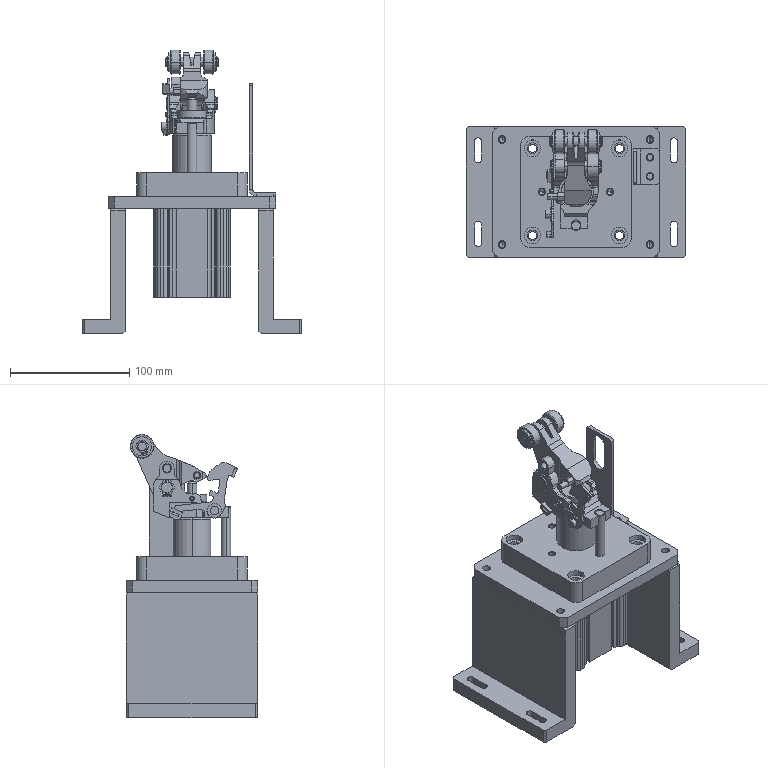Part | SolidWorks | features CompositeCurve 2 | 7 solids | 703 faces | box 184 x 110 x 237.505 mm | volume 955492 mm3 | plane 327 | cylinder 313 | cone 62 | spline 1 | commonest cylinder face diameters 2 x49 8 x35 6 x23 10 x16 14 x16 5 x14